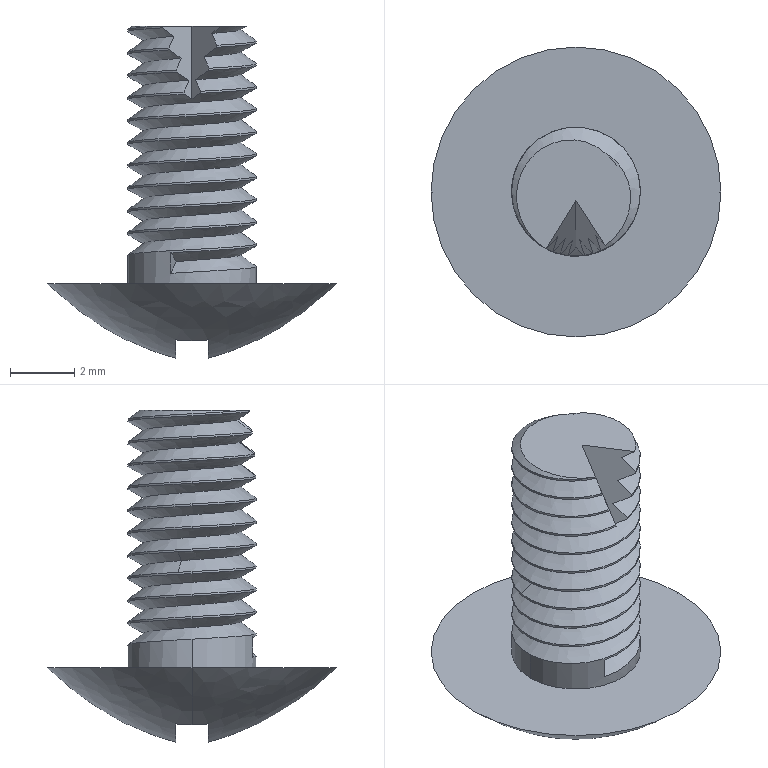Part | STEP file | 1 solid | 55 faces | box 9 x 9 x 10.31 mm | volume 144.628 mm3 | cylinder 23 | plane 18 | spline 14 | commonest cylinder face diameters 4 x23